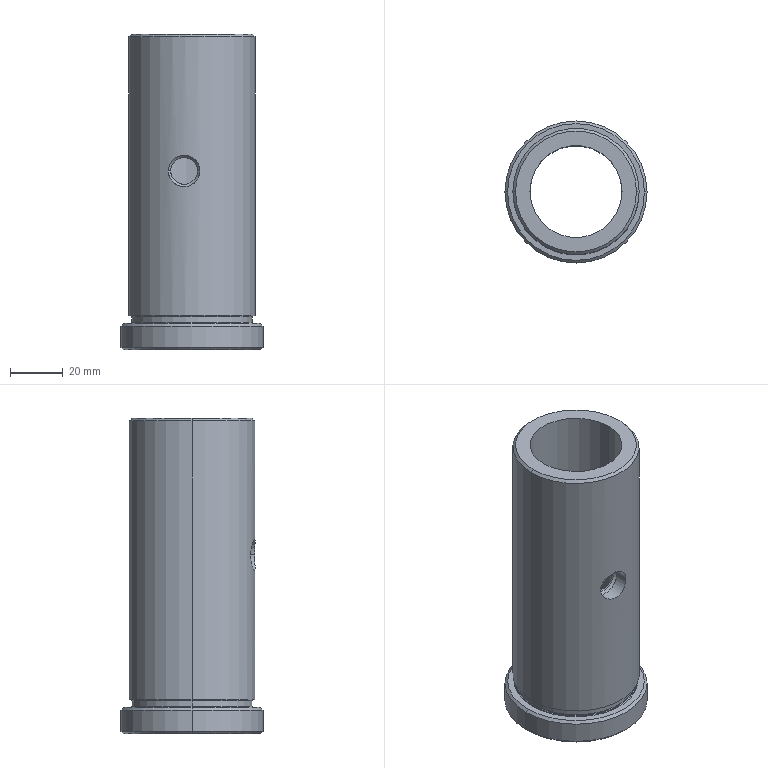Part | Creo | 1 solid | 32 faces | box 54 x 54 x 120 mm | volume 105135 mm3 | cylinder 12 | cone 8 | torus 8 | plane 4 | commonest cylinder face diameters 10.2 x2 12 x2 35 x2 46 x2 48 x2 54 x2
STEP:
#1=CARTESIAN_POINT('',(0.,0.,0.));
#2=DIRECTION('',(0.,0.,1.));
#3=DIRECTION('',(1.,0.,0.));
#4=AXIS2_PLACEMENT_3D('',#1,#2,#3);
#5=CARTESIAN_POINT('',(-189.,-212.,-111.5));
#6=VERTEX_POINT('',#5);
#7=CARTESIAN_POINT('',(-135.,-212.,-111.5));
#8=VERTEX_POINT('',#7);
#9=CARTESIAN_POINT('',(-162.,-212.,-111.5));
#10=DIRECTION('',(0.,0.,1.));
#11=DIRECTION('',(-1.,0.,0.));
#12=AXIS2_PLACEMENT_3D('',#9,#10,#11);
#13=CIRCLE('',#12,27.);
#14=EDGE_CURVE('',#6,#8,#13,.T.);
#15=ORIENTED_EDGE('',*,*,#14,.T.);
#16=CARTESIAN_POINT('',(-135.,-212.,-119.5));
#17=VERTEX_POINT('',#16);
#18=CARTESIAN_POINT('',(-135.,-212.,-111.5));
#19=DIRECTION('',(0.,0.,-1.));
#20=VECTOR('',#19,8.);
#21=LINE('',#18,#20);
#22=EDGE_CURVE('',#8,#17,#21,.T.);
#23=ORIENTED_EDGE('',*,*,#22,.T.);
#24=CARTESIAN_POINT('',(-189.,-212.,-119.5));
#25=VERTEX_POINT('',#24);
#26=CARTESIAN_POINT('',(-162.,-212.,-119.5));
#27=DIRECTION('',(0.,0.,-1.));
#28=DIRECTION('',(1.,0.,0.));
#29=AXIS2_PLACEMENT_3D('',#26,#27,#28);
#30=CIRCLE('',#29,27.);
#31=EDGE_CURVE('',#17,#25,#30,.T.);
#32=ORIENTED_EDGE('',*,*,#31,.T.);
#33=CARTESIAN_POINT('',(-189.,-212.,-111.5));
#34=DIRECTION('',(0.,0.,-1.));
#35=VECTOR('',#34,8.);
#36=LINE('',#33,#35);
#37=EDGE_CURVE('',#6,#25,#36,.T.);
#38=ORIENTED_EDGE('',*,*,#37,.F.);
#39=EDGE_LOOP('',(#15,#23,#32,#38));
#40=FACE_OUTER_BOUND('',#39,.F.);
#41=CARTESIAN_POINT('',(-162.,-212.,-110.5));
#42=DIRECTION('',(0.,0.,-1.));
#43=DIRECTION('',(1.,0.,0.));
#44=AXIS2_PLACEMENT_3D('',#41,#42,#43);
#45=CYLINDRICAL_SURFACE('',#44,27.);
#46=ADVANCED_FACE('',(#40),#45,.T.);
#47=CARTESIAN_POINT('',(-188.,-212.,-110.5));
#48=VERTEX_POINT('',#47);
#49=CARTESIAN_POINT('',(-136.,-212.,-110.5));
#50=VERTEX_POINT('',#49);
#51=CARTESIAN_POINT('',(-162.,-212.,-110.5));
#52=DIRECTION('',(0.,0.,1.));
#53=DIRECTION('',(-1.,0.,0.));
#54=AXIS2_PLACEMENT_3D('',#51,#52,#53);
#55=CIRCLE('',#54,26.);
#56=EDGE_CURVE('',#48,#50,#55,.T.);
#57=ORIENTED_EDGE('',*,*,#56,.T.);
#58=CARTESIAN_POINT('',(-136.,-212.,-110.5));
#59=DIRECTION('',(0.7071,0.,-0.7071));
#60=VECTOR('',#59,1.414);
#61=LINE('',#58,#60);
#62=EDGE_CURVE('',#50,#8,#61,.T.);
#63=ORIENTED_EDGE('',*,*,#62,.T.);
#64=ORIENTED_EDGE('',*,*,#14,.F.);
#65=CARTESIAN_POINT('',(-188.,-212.,-110.5));
#66=DIRECTION('',(-0.7071,0.,-0.7071));
#67=VECTOR('',#66,1.414);
#68=LINE('',#65,#67);
#69=EDGE_CURVE('',#48,#6,#68,.T.);
#70=ORIENTED_EDGE('',*,*,#69,.F.);
#71=EDGE_LOOP('',(#57,#63,#64,#70));
#72=FACE_OUTER_BOUND('',#71,.F.);
#73=CARTESIAN_POINT('',(-162.,-212.,-111.));
#74=DIRECTION('',(0.,0.,-1.));
#75=DIRECTION('',(1.,0.,0.));
#76=AXIS2_PLACEMENT_3D('',#73,#74,#75);
#77=CONICAL_SURFACE('',#76,26.5,45.);
#78=ADVANCED_FACE('',(#72),#77,.T.);
#79=ORIENTED_EDGE('',*,*,#56,.F.);
#80=CARTESIAN_POINT('',(-162.,-212.,-110.5));
#81=DIRECTION('',(0.,0.,1.));
#82=DIRECTION('',(1.,0.,0.));
#83=AXIS2_PLACEMENT_3D('',#80,#81,#82);
#84=CIRCLE('',#83,26.);
#85=EDGE_CURVE('',#50,#48,#84,.T.);
#86=ORIENTED_EDGE('',*,*,#85,.F.);
#87=EDGE_LOOP('',(#79,#86));
#88=FACE_OUTER_BOUND('',#87,.F.);
#89=CARTESIAN_POINT('',(-138.5,-212.,-110.5));
#90=VERTEX_POINT('',#89);
#91=CARTESIAN_POINT('',(-185.5,-212.,-110.5));
#92=VERTEX_POINT('',#91);
#93=CARTESIAN_POINT('',(-162.,-212.,-110.5));
#94=DIRECTION('',(0.,0.,-1.));
#95=DIRECTION('',(1.,0.,0.));
#96=AXIS2_PLACEMENT_3D('',#93,#94,#95);
#97=CIRCLE('',#96,23.5);
#98=EDGE_CURVE('',#90,#92,#97,.T.);
#99=ORIENTED_EDGE('',*,*,#98,.F.);
#100=CARTESIAN_POINT('',(-162.,-212.,-110.5));
#101=DIRECTION('',(0.,0.,-1.));
#102=DIRECTION('',(-1.,0.,0.));
#103=AXIS2_PLACEMENT_3D('',#100,#101,#102);
#104=CIRCLE('',#103,23.5);
#105=EDGE_CURVE('',#92,#90,#104,.T.);
#106=ORIENTED_EDGE('',*,*,#105,.F.);
#107=EDGE_LOOP('',(#99,#106));
#108=FACE_BOUND('',#107,.F.);
#109=CARTESIAN_POINT('',(-162.,-212.,-110.5));
#110=DIRECTION('',(0.,0.,-1.));
#111=DIRECTION('',(1.,0.,0.));
#112=AXIS2_PLACEMENT_3D('',#109,#110,#111);
#113=PLANE('',#112);
#114=ADVANCED_FACE('',(#88,#108),#113,.F.);
#115=ORIENTED_EDGE('',*,*,#85,.T.);
#116=ORIENTED_EDGE('',*,*,#69,.T.);
#117=CARTESIAN_POINT('',(-162.,-212.,-111.5));
#118=DIRECTION('',(0.,0.,1.));
#119=DIRECTION('',(1.,0.,0.));
#120=AXIS2_PLACEMENT_3D('',#117,#118,#119);
#121=CIRCLE('',#120,27.);
#122=EDGE_CURVE('',#8,#6,#121,.T.);
#123=ORIENTED_EDGE('',*,*,#122,.F.);
#124=ORIENTED_EDGE('',*,*,#62,.F.);
#125=EDGE_LOOP('',(#115,#116,#123,#124));
#126=FACE_OUTER_BOUND('',#125,.F.);
#127=CARTESIAN_POINT('',(-162.,-212.,-111.));
#128=DIRECTION('',(0.,0.,-1.));
#129=DIRECTION('',(1.,0.,0.));
#130=AXIS2_PLACEMENT_3D('',#127,#128,#129);
#131=CONICAL_SURFACE('',#130,26.5,45.);
#132=ADVANCED_FACE('',(#126),#131,.T.);
#133=ORIENTED_EDGE('',*,*,#122,.T.);
#134=ORIENTED_EDGE('',*,*,#37,.T.);
#135=CARTESIAN_POINT('',(-162.,-212.,-119.5));
#136=DIRECTION('',(0.,0.,-1.));
#137=DIRECTION('',(-1.,0.,0.));
#138=AXIS2_PLACEMENT_3D('',#135,#136,#137);
#139=CIRCLE('',#138,27.);
#140=EDGE_CURVE('',#25,#17,#139,.T.);
#141=ORIENTED_EDGE('',*,*,#140,.T.);
#142=ORIENTED_EDGE('',*,*,#22,.F.);
#143=EDGE_LOOP('',(#133,#134,#141,#142));
#144=FACE_OUTER_BOUND('',#143,.F.);
#145=CARTESIAN_POINT('',(-162.,-212.,-110.5));
#146=DIRECTION('',(0.,0.,-1.));
#147=DIRECTION('',(1.,0.,0.));
#148=AXIS2_PLACEMENT_3D('',#145,#146,#147);
#149=CYLINDRICAL_SURFACE('',#148,27.);
#150=ADVANCED_FACE('',(#144),#149,.T.);
#151=ORIENTED_EDGE('',*,*,#140,.F.);
#152=CARTESIAN_POINT('',(-188.,-212.,-120.5));
#153=VERTEX_POINT('',#152);
#154=CARTESIAN_POINT('',(-188.,-212.,-120.5));
#155=DIRECTION('',(-0.7071,0.,0.7071));
#156=VECTOR('',#155,1.414);
#157=LINE('',#154,#156);
#158=EDGE_CURVE('',#153,#25,#157,.T.);
#159=ORIENTED_EDGE('',*,*,#158,.F.);
#160=CARTESIAN_POINT('',(-136.,-212.,-120.5));
#161=VERTEX_POINT('',#160);
#162=CARTESIAN_POINT('',(-162.,-212.,-120.5));
#163=DIRECTION('',(0.,0.,-1.));
#164=DIRECTION('',(-1.,0.,0.));
#165=AXIS2_PLACEMENT_3D('',#162,#163,#164);
#166=CIRCLE('',#165,26.);
#167=EDGE_CURVE('',#153,#161,#166,.T.);
#168=ORIENTED_EDGE('',*,*,#167,.T.);
#169=CARTESIAN_POINT('',(-136.,-212.,-120.5));
#170=DIRECTION('',(0.7071,0.,0.7071));
#171=VECTOR('',#170,1.414);
#172=LINE('',#169,#171);
#173=EDGE_CURVE('',#161,#17,#172,.T.);
#174=ORIENTED_EDGE('',*,*,#173,.T.);
#175=EDGE_LOOP('',(#151,#159,#168,#174));
#176=FACE_OUTER_BOUND('',#175,.F.);
#177=CARTESIAN_POINT('',(-162.,-212.,-120.));
#178=DIRECTION('',(0.,0.,1.));
#179=DIRECTION('',(-1.,0.,0.));
#180=AXIS2_PLACEMENT_3D('',#177,#178,#179);
#181=CONICAL_SURFACE('',#180,26.5,45.);
#182=ADVANCED_FACE('',(#176),#181,.T.);
#183=ORIENTED_EDGE('',*,*,#31,.F.);
#184=ORIENTED_EDGE('',*,*,#173,.F.);
#185=CARTESIAN_POINT('',(-162.,-212.,-120.5));
#186=DIRECTION('',(0.,0.,-1.));
#187=DIRECTION('',(1.,0.,0.));
#188=AXIS2_PLACEMENT_3D('',#185,#186,#187);
#189=CIRCLE('',#188,26.);
#190=EDGE_CURVE('',#161,#153,#189,.T.);
#191=ORIENTED_EDGE('',*,*,#190,.T.);
#192=ORIENTED_EDGE('',*,*,#158,.T.);
#193=EDGE_LOOP('',(#183,#184,#191,#192));
#194=FACE_OUTER_BOUND('',#193,.F.);
#195=CARTESIAN_POINT('',(-162.,-212.,-120.));
#196=DIRECTION('',(0.,0.,1.));
#197=DIRECTION('',(-1.,0.,0.));
#198=AXIS2_PLACEMENT_3D('',#195,#196,#197);
#199=CONICAL_SURFACE('',#198,26.5,45.);
#200=ADVANCED_FACE('',(#194),#199,.T.);
#201=ORIENTED_EDGE('',*,*,#167,.F.);
#202=ORIENTED_EDGE('',*,*,#190,.F.);
#203=EDGE_LOOP('',(#201,#202));
#204=FACE_OUTER_BOUND('',#203,.F.);
#205=CARTESIAN_POINT('',(-144.5,-212.,-120.5));
#206=VERTEX_POINT('',#205);
#207=CARTESIAN_POINT('',(-179.5,-212.,-120.5));
#208=VERTEX_POINT('',#207);
#209=CARTESIAN_POINT('',(-162.,-212.,-120.5));
#210=DIRECTION('',(0.,0.,1.));
#211=DIRECTION('',(1.,0.,0.));
#212=AXIS2_PLACEMENT_3D('',#209,#210,#211);
#213=CIRCLE('',#212,17.5);
#214=EDGE_CURVE('',#206,#208,#213,.T.);
#215=ORIENTED_EDGE('',*,*,#214,.F.);
#216=CARTESIAN_POINT('',(-162.,-212.,-120.5));
#217=DIRECTION('',(0.,0.,1.));
#218=DIRECTION('',(-1.,0.,0.));
#219=AXIS2_PLACEMENT_3D('',#216,#217,#218);
#220=CIRCLE('',#219,17.5);
#221=EDGE_CURVE('',#208,#206,#220,.T.);
#222=ORIENTED_EDGE('',*,*,#221,.F.);
#223=EDGE_LOOP('',(#215,#222));
#224=FACE_BOUND('',#223,.F.);
#225=CARTESIAN_POINT('',(-162.,-212.,-120.5));
#226=DIRECTION('',(0.,0.,-1.));
#227=DIRECTION('',(1.,0.,0.));
#228=AXIS2_PLACEMENT_3D('',#225,#226,#227);
#229=PLANE('',#228);
#230=ADVANCED_FACE('',(#204,#224),#229,.T.);
#231=CARTESIAN_POINT('',(-179.5,-212.,-0.5));
#232=VERTEX_POINT('',#231);
#233=CARTESIAN_POINT('',(-144.5,-212.,-0.5));
#234=VERTEX_POINT('',#233);
#235=CARTESIAN_POINT('',(-162.,-212.,-0.5));
#236=DIRECTION('',(0.,0.,-1.));
#237=DIRECTION('',(-1.,0.,0.));
#238=AXIS2_PLACEMENT_3D('',#235,#236,#237);
#239=CIRCLE('',#238,17.5);
#240=EDGE_CURVE('',#232,#234,#239,.T.);
#241=ORIENTED_EDGE('',*,*,#240,.T.);
#242=CARTESIAN_POINT('',(-144.5,-212.,-120.5));
#243=DIRECTION('',(0.,0.,1.));
#244=VECTOR('',#243,120.);
#245=LINE('',#242,#244);
#246=EDGE_CURVE('',#206,#234,#245,.T.);
#247=ORIENTED_EDGE('',*,*,#246,.F.);
#248=ORIENTED_EDGE('',*,*,#214,.T.);
#249=CARTESIAN_POINT('',(-179.5,-212.,-120.5));
#250=DIRECTION('',(0.,0.,1.));
#251=VECTOR('',#250,120.);
#252=LINE('',#249,#251);
#253=EDGE_CURVE('',#208,#232,#252,.T.);
#254=ORIENTED_EDGE('',*,*,#253,.T.);
#255=EDGE_LOOP('',(#241,#247,#248,#254));
#256=FACE_OUTER_BOUND('',#255,.F.);
#257=CARTESIAN_POINT('',(-162.,-212.,-120.5));
#258=DIRECTION('',(0.,0.,1.));
#259=DIRECTION('',(-1.,0.,0.));
#260=AXIS2_PLACEMENT_3D('',#257,#258,#259);
#261=CYLINDRICAL_SURFACE('',#260,17.5);
#262=ADVANCED_FACE('',(#256),#261,.F.);
#263=CARTESIAN_POINT('',(-139.,-212.,-0.5));
#264=VERTEX_POINT('',#263);
#265=CARTESIAN_POINT('',(-185.,-212.,-0.5));
#266=VERTEX_POINT('',#265);
#267=CARTESIAN_POINT('',(-162.,-212.,-0.5));
#268=DIRECTION('',(0.,0.,1.));
#269=DIRECTION('',(1.,0.,0.));
#270=AXIS2_PLACEMENT_3D('',#267,#268,#269);
#271=CIRCLE('',#270,23.);
#272=EDGE_CURVE('',#264,#266,#271,.T.);
#273=ORIENTED_EDGE('',*,*,#272,.F.);
#274=CARTESIAN_POINT('',(-162.,-212.,-0.5));
#275=DIRECTION('',(0.,0.,1.));
#276=DIRECTION('',(-1.,0.,0.));
#277=AXIS2_PLACEMENT_3D('',#274,#275,#276);
#278=CIRCLE('',#277,23.);
#279=EDGE_CURVE('',#266,#264,#278,.T.);
#280=ORIENTED_EDGE('',*,*,#279,.F.);
#281=EDGE_LOOP('',(#273,#280));
#282=FACE_OUTER_BOUND('',#281,.F.);
#283=CARTESIAN_POINT('',(-162.,-212.,-0.5));
#284=DIRECTION('',(0.,0.,-1.));
#285=DIRECTION('',(1.,0.,0.));
#286=AXIS2_PLACEMENT_3D('',#283,#284,#285);
#287=CIRCLE('',#286,17.5);
#288=EDGE_CURVE('',#234,#232,#287,.T.);
#289=ORIENTED_EDGE('',*,*,#288,.F.);
#290=ORIENTED_EDGE('',*,*,#240,.F.);
#291=EDGE_LOOP('',(#289,#290));
#292=FACE_BOUND('',#291,.F.);
#293=CARTESIAN_POINT('',(-162.,-212.,-0.5));
#294=DIRECTION('',(0.,0.,1.));
#295=DIRECTION('',(-1.,0.,0.));
#296=AXIS2_PLACEMENT_3D('',#293,#294,#295);
#297=PLANE('',#296);
#298=ADVANCED_FACE('',(#282,#292),#297,.T.);
#299=ORIENTED_EDGE('',*,*,#288,.T.);
#300=ORIENTED_EDGE('',*,*,#253,.F.);
#301=ORIENTED_EDGE('',*,*,#221,.T.);
#302=ORIENTED_EDGE('',*,*,#246,.T.);
#303=EDGE_LOOP('',(#299,#300,#301,#302));
#304=FACE_OUTER_BOUND('',#303,.F.);
#305=CARTESIAN_POINT('',(-159.9,-229.374,-52.5));
#306=VERTEX_POINT('',#305);
#307=CARTESIAN_POINT('',(-170.1,-227.513,-52.5));
#308=VERTEX_POINT('',#307);
#309=CARTESIAN_POINT('',(-159.9,-229.374,-52.5));
#310=CARTESIAN_POINT('',(-159.9,-229.374,-52.883));
#311=CARTESIAN_POINT('',(-159.986,-229.384,-53.65));
#312=CARTESIAN_POINT('',(-160.375,-229.427,-54.754));
#313=CARTESIAN_POINT('',(-161.008,-229.477,-55.743));
#314=CARTESIAN_POINT('',(-161.827,-229.507,-56.548));
#315=CARTESIAN_POINT('',(-162.814,-229.492,-57.156));
#316=CARTESIAN_POINT('',(-163.903,-229.408,-57.524));
#317=CARTESIAN_POINT('',(-165.043,-229.246,-57.642));
#318=CARTESIAN_POINT('',(-166.188,-229.005,-57.505));
#319=CARTESIAN_POINT('',(-167.292,-228.693,-57.107));
#320=CARTESIAN_POINT('',(-168.281,-228.344,-56.462));
#321=CARTESIAN_POINT('',(-169.086,-228.007,-55.625));
#322=CARTESIAN_POINT('',(-169.686,-227.725,-54.621));
#323=CARTESIAN_POINT('',(-170.032,-227.549,-53.544));
#324=CARTESIAN_POINT('',(-170.1,-227.513,-52.841));
#325=CARTESIAN_POINT('',(-170.1,-227.513,-52.5));
#326=B_SPLINE_CURVE_WITH_KNOTS('',3,(#309,#310,#311,#312,#313,#314,#315,#316,#317,#318,#319,#320,#321,#322,#323,#324,#325),.UNSPECIFIED.,.F.,.F.,(4,1,1,1,1,1,1,1,1,1,1,1,1,1,4),(0.,0.07143,0.1429,0.2143,0.2857,0.3571,0.4286,0.5,0.5714,0.6429,0.7143,0.7857,0.8571,0.9286,1.),.UNSPECIFIED.);
#327=EDGE_CURVE('',#306,#308,#326,.T.);
#328=ORIENTED_EDGE('',*,*,#327,.T.);
#329=CARTESIAN_POINT('',(-170.1,-227.513,-52.5));
#330=CARTESIAN_POINT('',(-170.1,-227.513,-52.158));
#331=CARTESIAN_POINT('',(-170.031,-227.549,-51.456));
#332=CARTESIAN_POINT('',(-169.689,-227.723,-50.388));
#333=CARTESIAN_POINT('',(-169.099,-228.001,-49.393));
#334=CARTESIAN_POINT('',(-168.303,-228.335,-48.556));
#335=CARTESIAN_POINT('',(-167.317,-228.685,-47.905));
#336=CARTESIAN_POINT('',(-166.207,-229.,-47.499));
#337=CARTESIAN_POINT('',(-165.06,-229.244,-47.358));
#338=CARTESIAN_POINT('',(-163.922,-229.406,-47.472));
#339=CARTESIAN_POINT('',(-162.838,-229.49,-47.834));
#340=CARTESIAN_POINT('',(-161.851,-229.507,-48.434));
#341=CARTESIAN_POINT('',(-161.022,-229.478,-49.239));
#342=CARTESIAN_POINT('',(-160.38,-229.427,-50.234));
#343=CARTESIAN_POINT('',(-159.986,-229.384,-51.349));
#344=CARTESIAN_POINT('',(-159.9,-229.374,-52.119));
#345=CARTESIAN_POINT('',(-159.9,-229.374,-52.5));
#346=B_SPLINE_CURVE_WITH_KNOTS('',3,(#329,#330,#331,#332,#333,#334,#335,#336,#337,#338,#339,#340,#341,#342,#343,#344,#345),.UNSPECIFIED.,.F.,.F.,(4,1,1,1,1,1,1,1,1,1,1,1,1,1,4),(0.,0.07143,0.1429,0.2143,0.2857,0.3571,0.4286,0.5,0.5714,0.6429,0.7143,0.7857,0.8571,0.9286,1.),.UNSPECIFIED.);
#347=EDGE_CURVE('',#308,#306,#346,.T.);
#348=ORIENTED_EDGE('',*,*,#347,.T.);
#349=EDGE_LOOP('',(#328,#348));
#350=FACE_BOUND('',#349,.F.);
#351=CARTESIAN_POINT('',(-162.,-212.,-120.5));
#352=DIRECTION('',(0.,0.,1.));
#353=DIRECTION('',(-1.,0.,0.));
#354=AXIS2_PLACEMENT_3D('',#351,#352,#353);
#355=CYLINDRICAL_SURFACE('',#354,17.5);
#356=ADVANCED_FACE('',(#304,#350),#355,.F.);
#357=CARTESIAN_POINT('',(-159.9,-230.1,-52.5));
#358=VERTEX_POINT('',#357);
#359=CARTESIAN_POINT('',(-170.1,-230.1,-52.5));
#360=VERTEX_POINT('',#359);
#361=CARTESIAN_POINT('',(-165.,-230.1,-52.5));
#362=DIRECTION('',(0.,1.,0.));
#363=DIRECTION('',(1.,0.,0.));
#364=AXIS2_PLACEMENT_3D('',#361,#362,#363);
#365=CIRCLE('',#364,5.1);
#366=EDGE_CURVE('',#358,#360,#365,.T.);
#367=ORIENTED_EDGE('',*,*,#366,.T.);
#368=CARTESIAN_POINT('',(-170.1,-227.513,-52.5));
#369=DIRECTION('',(0.,-1.,0.));
#370=VECTOR('',#369,2.587);
#371=LINE('',#368,#370);
#372=EDGE_CURVE('',#308,#360,#371,.T.);
#373=ORIENTED_EDGE('',*,*,#372,.F.);
#374=ORIENTED_EDGE('',*,*,#327,.F.);
#375=CARTESIAN_POINT('',(-159.9,-229.374,-52.5));
#376=DIRECTION('',(0.00000007,-1.,0.000573));
#377=VECTOR('',#376,0.7265);
#378=LINE('',#375,#377);
#379=EDGE_CURVE('',#306,#358,#378,.T.);
#380=ORIENTED_EDGE('',*,*,#379,.T.);
#381=EDGE_LOOP('',(#367,#373,#374,#380));
#382=FACE_OUTER_BOUND('',#381,.F.);
#383=CARTESIAN_POINT('',(-165.,-300.,-52.5));
#384=DIRECTION('',(0.,-1.,0.));
#385=DIRECTION('',(-1.,0.,0.));
#386=AXIS2_PLACEMENT_3D('',#383,#384,#385);
#387=CYLINDRICAL_SURFACE('',#386,5.1);
#388=ADVANCED_FACE('',(#382),#387,.F.);
#389=ORIENTED_EDGE('',*,*,#366,.F.);
#390=CARTESIAN_POINT('',(-159.,-231.,-52.5));
#391=VERTEX_POINT('',#390);
#392=CARTESIAN_POINT('',(-159.9,-230.1,-52.5));
#393=DIRECTION('',(0.7071,-0.7071,0.));
#394=VECTOR('',#393,1.273);
#395=LINE('',#392,#394);
#396=EDGE_CURVE('',#358,#391,#395,.T.);
#397=ORIENTED_EDGE('',*,*,#396,.T.);
#398=CARTESIAN_POINT('',(-171.,-231.,-52.5));
#399=VERTEX_POINT('',#398);
#400=CARTESIAN_POINT('',(-165.,-231.,-52.5));
#401=DIRECTION('',(0.,-1.,0.));
#402=DIRECTION('',(-1.,0.,0.));
#403=AXIS2_PLACEMENT_3D('',#400,#401,#402);
#404=CIRCLE('',#403,6.);
#405=EDGE_CURVE('',#399,#391,#404,.T.);
#406=ORIENTED_EDGE('',*,*,#405,.F.);
#407=CARTESIAN_POINT('',(-170.1,-230.1,-52.5));
#408=DIRECTION('',(-0.7071,-0.7071,0.));
#409=VECTOR('',#408,1.273);
#410=LINE('',#407,#409);
#411=EDGE_CURVE('',#360,#399,#410,.T.);
#412=ORIENTED_EDGE('',*,*,#411,.F.);
#413=EDGE_LOOP('',(#389,#397,#406,#412));
#414=FACE_OUTER_BOUND('',#413,.F.);
#415=CARTESIAN_POINT('',(-165.,-230.55,-52.5));
#416=DIRECTION('',(0.,-1.,0.));
#417=DIRECTION('',(-1.,0.,0.));
#418=AXIS2_PLACEMENT_3D('',#415,#416,#417);
#419=CONICAL_SURFACE('',#418,5.55,45.);
#420=ADVANCED_FACE('',(#414),#419,.F.);
#421=CARTESIAN_POINT('',(-165.,-230.1,-52.5));
#422=DIRECTION('',(0.,1.,0.));
#423=DIRECTION('',(-1.,0.,0.));
#424=AXIS2_PLACEMENT_3D('',#421,#422,#423);
#425=CIRCLE('',#424,5.1);
#426=EDGE_CURVE('',#360,#358,#425,.T.);
#427=ORIENTED_EDGE('',*,*,#426,.F.);
#428=ORIENTED_EDGE('',*,*,#411,.T.);
#429=CARTESIAN_POINT('',(-165.,-231.,-52.5));
#430=DIRECTION('',(0.,-1.,0.));
#431=DIRECTION('',(1.,0.,0.));
#432=AXIS2_PLACEMENT_3D('',#429,#430,#431);
#433=CIRCLE('',#432,6.);
#434=EDGE_CURVE('',#391,#399,#433,.T.);
#435=ORIENTED_EDGE('',*,*,#434,.F.);
#436=ORIENTED_EDGE('',*,*,#396,.F.);
#437=EDGE_LOOP('',(#427,#428,#435,#436));
#438=FACE_OUTER_BOUND('',#437,.F.);
#439=CARTESIAN_POINT('',(-165.,-230.55,-52.5));
#440=DIRECTION('',(0.,-1.,0.));
#441=DIRECTION('',(-1.,0.,0.));
#442=AXIS2_PLACEMENT_3D('',#439,#440,#441);
#443=CONICAL_SURFACE('',#442,5.55,45.);
#444=ADVANCED_FACE('',(#438),#443,.F.);
#445=ORIENTED_EDGE('',*,*,#426,.T.);
#446=ORIENTED_EDGE('',*,*,#379,.F.);
#447=ORIENTED_EDGE('',*,*,#347,.F.);
#448=ORIENTED_EDGE('',*,*,#372,.T.);
#449=EDGE_LOOP('',(#445,#446,#447,#448));
#450=FACE_OUTER_BOUND('',#449,.F.);
#451=CARTESIAN_POINT('',(-165.,-300.,-52.5));
#452=DIRECTION('',(0.,-1.,0.));
#453=DIRECTION('',(-1.,0.,0.));
#454=AXIS2_PLACEMENT_3D('',#451,#452,#453);
#455=CYLINDRICAL_SURFACE('',#454,5.1);
#456=ADVANCED_FACE('',(#450),#455,.F.);
#457=CARTESIAN_POINT('',(-171.,-234.249,-52.5));
#458=VERTEX_POINT('',#457);
#459=CARTESIAN_POINT('',(-159.,-235.812,-52.501));
#460=VERTEX_POINT('',#459);
#461=CARTESIAN_POINT('',(-171.,-234.249,-52.5));
#462=CARTESIAN_POINT('',(-171.,-234.249,-52.07));
#463=CARTESIAN_POINT('',(-170.911,-234.285,-51.222));
#464=CARTESIAN_POINT('',(-170.485,-234.453,-49.943));
#465=CARTESIAN_POINT('',(-169.772,-234.713,-48.779));
#466=CARTESIAN_POINT('',(-168.819,-235.02,-47.806));
#467=CARTESIAN_POINT('',(-167.66,-235.335,-47.063));
#468=CARTESIAN_POINT('',(-166.358,-235.614,-46.602));
#469=CARTESIAN_POINT('',(-164.999,-235.825,-46.449));
#470=CARTESIAN_POINT('',(-163.646,-235.956,-46.603));
#471=CARTESIAN_POINT('',(-162.366,-236.008,-47.053));
#472=CARTESIAN_POINT('',(-161.221,-235.995,-47.776));
#473=CARTESIAN_POINT('',(-160.271,-235.943,-48.726));
#474=CARTESIAN_POINT('',(-159.544,-235.876,-49.88));
#475=CARTESIAN_POINT('',(-159.098,-235.824,-51.173));
#476=CARTESIAN_POINT('',(-159.,-235.812,-52.05));
#477=CARTESIAN_POINT('',(-159.,-235.812,-52.501));
#478=B_SPLINE_CURVE_WITH_KNOTS('',3,(#461,#462,#463,#464,#465,#466,#467,#468,#469,#470,#471,#472,#473,#474,#475,#476,#477),.UNSPECIFIED.,.F.,.F.,(4,1,1,1,1,1,1,1,1,1,1,1,1,1,4),(0.,0.07143,0.1429,0.2143,0.2857,0.3571,0.4286,0.5,0.5714,0.6429,0.7143,0.7857,0.8571,0.9286,1.),.UNSPECIFIED.);
#479=EDGE_CURVE('',#458,#460,#478,.T.);
#480=ORIENTED_EDGE('',*,*,#479,.T.);
#481=CARTESIAN_POINT('',(-159.,-231.,-52.5));
#482=DIRECTION('',(-0.000000014,-1.,-0.0001098));
#483=VECTOR('',#482,4.812);
#484=LINE('',#481,#483);
#485=EDGE_CURVE('',#391,#460,#484,.T.);
#486=ORIENTED_EDGE('',*,*,#485,.F.);
#487=ORIENTED_EDGE('',*,*,#434,.T.);
#488=CARTESIAN_POINT('',(-171.,-231.,-52.5));
#489=DIRECTION('',(0.,-1.,0.));
#490=VECTOR('',#489,3.249);
#491=LINE('',#488,#490);
#492=EDGE_CURVE('',#399,#458,#491,.T.);
#493=ORIENTED_EDGE('',*,*,#492,.T.);
#494=EDGE_LOOP('',(#480,#486,#487,#493));
#495=FACE_OUTER_BOUND('',#494,.F.);
#496=CARTESIAN_POINT('',(-165.,-300.,-52.5));
#497=DIRECTION('',(0.,-1.,0.));
#498=DIRECTION('',(-1.,0.,0.));
#499=AXIS2_PLACEMENT_3D('',#496,#497,#498);
#500=CYLINDRICAL_SURFACE('',#499,6.);
#501=ADVANCED_FACE('',(#495),#500,.F.);
#502=CARTESIAN_POINT('',(-138.,-212.,-107.5));
#503=VERTEX_POINT('',#502);
#504=CARTESIAN_POINT('',(-186.,-212.,-107.5));
#505=VERTEX_POINT('',#504);
#506=CARTESIAN_POINT('',(-162.,-212.,-107.5));
#507=DIRECTION('',(0.,0.,-1.));
#508=DIRECTION('',(1.,0.,0.));
#509=AXIS2_PLACEMENT_3D('',#506,#507,#508);
#510=CIRCLE('',#509,24.);
#511=EDGE_CURVE('',#503,#505,#510,.T.);
#512=ORIENTED_EDGE('',*,*,#511,.T.);
#513=CARTESIAN_POINT('',(-186.,-212.,-1.5));
#514=VERTEX_POINT('',#513);
#515=CARTESIAN_POINT('',(-186.,-212.,-107.5));
#516=DIRECTION('',(0.,0.,1.));
#517=VECTOR('',#516,106.);
#518=LINE('',#515,#517);
#519=EDGE_CURVE('',#505,#514,#518,.T.);
#520=ORIENTED_EDGE('',*,*,#519,.T.);
#521=CARTESIAN_POINT('',(-138.,-212.,-1.5));
#522=VERTEX_POINT('',#521);
#523=CARTESIAN_POINT('',(-162.,-212.,-1.5));
#524=DIRECTION('',(0.,0.,1.));
#525=DIRECTION('',(-1.,0.,0.));
#526=AXIS2_PLACEMENT_3D('',#523,#524,#525);
#527=CIRCLE('',#526,24.);
#528=EDGE_CURVE('',#514,#522,#527,.T.);
#529=ORIENTED_EDGE('',*,*,#528,.T.);
#530=CARTESIAN_POINT('',(-138.,-212.,-107.5));
#531=DIRECTION('',(0.,0.,1.));
#532=VECTOR('',#531,106.);
#533=LINE('',#530,#532);
#534=EDGE_CURVE('',#503,#522,#533,.T.);
#535=ORIENTED_EDGE('',*,*,#534,.F.);
#536=EDGE_LOOP('',(#512,#520,#529,#535));
#537=FACE_OUTER_BOUND('',#536,.F.);
#538=ORIENTED_EDGE('',*,*,#479,.F.);
#539=CARTESIAN_POINT('',(-159.,-235.812,-52.501));
#540=CARTESIAN_POINT('',(-159.,-235.812,-52.95));
#541=CARTESIAN_POINT('',(-159.099,-235.824,-53.828));
#542=CARTESIAN_POINT('',(-159.539,-235.876,-55.107));
#543=CARTESIAN_POINT('',(-160.258,-235.942,-56.257));
#544=CARTESIAN_POINT('',(-161.198,-235.994,-57.206));
#545=CARTESIAN_POINT('',(-162.349,-236.008,-57.94));
#546=CARTESIAN_POINT('',(-163.632,-235.957,-58.394));
#547=CARTESIAN_POINT('',(-164.985,-235.827,-58.551));
#548=CARTESIAN_POINT('',(-166.34,-235.617,-58.401));
#549=CARTESIAN_POINT('',(-167.637,-235.34,-57.948));
#550=CARTESIAN_POINT('',(-168.801,-235.025,-57.209));
#551=CARTESIAN_POINT('',(-169.761,-234.716,-56.236));
#552=CARTESIAN_POINT('',(-170.481,-234.454,-55.066));
#553=CARTESIAN_POINT('',(-170.911,-234.285,-53.779));
#554=CARTESIAN_POINT('',(-171.,-234.249,-52.93));
#555=CARTESIAN_POINT('',(-171.,-234.249,-52.5));
#556=B_SPLINE_CURVE_WITH_KNOTS('',3,(#539,#540,#541,#542,#543,#544,#545,#546,#547,#548,#549,#550,#551,#552,#553,#554,#555),.UNSPECIFIED.,.F.,.F.,(4,1,1,1,1,1,1,1,1,1,1,1,1,1,4),(0.,0.07143,0.1429,0.2143,0.2857,0.3571,0.4286,0.5,0.5714,0.6429,0.7143,0.7857,0.8571,0.9286,1.),.UNSPECIFIED.);
#557=EDGE_CURVE('',#460,#458,#556,.T.);
#558=ORIENTED_EDGE('',*,*,#557,.F.);
#559=EDGE_LOOP('',(#538,#558));
#560=FACE_BOUND('',#559,.F.);
#561=CARTESIAN_POINT('',(-162.,-212.,-110.5));
#562=DIRECTION('',(0.,0.,1.));
#563=DIRECTION('',(-1.,0.,0.));
#564=AXIS2_PLACEMENT_3D('',#561,#562,#563);
#565=CYLINDRICAL_SURFACE('',#564,24.);
#566=ADVANCED_FACE('',(#537,#560),#565,.T.);
#567=ORIENTED_EDGE('',*,*,#557,.T.);
#568=ORIENTED_EDGE('',*,*,#492,.F.);
#569=ORIENTED_EDGE('',*,*,#405,.T.);
#570=ORIENTED_EDGE('',*,*,#485,.T.);
#571=EDGE_LOOP('',(#567,#568,#569,#570));
#572=FACE_OUTER_BOUND('',#571,.F.);
#573=CARTESIAN_POINT('',(-165.,-300.,-52.5));
#574=DIRECTION('',(0.,-1.,0.));
#575=DIRECTION('',(-1.,0.,0.));
#576=AXIS2_PLACEMENT_3D('',#573,#574,#575);
#577=CYLINDRICAL_SURFACE('',#576,6.);
#578=ADVANCED_FACE('',(#572),#577,.F.);
#579=ORIENTED_EDGE('',*,*,#511,.F.);
#580=CARTESIAN_POINT('',(-162.,-212.,-107.5));
#581=DIRECTION('',(0.,0.,-1.));
#582=DIRECTION('',(-1.,0.,0.));
#583=AXIS2_PLACEMENT_3D('',#580,#581,#582);
#584=CIRCLE('',#583,24.);
#585=EDGE_CURVE('',#505,#503,#584,.T.);
#586=ORIENTED_EDGE('',*,*,#585,.F.);
#587=EDGE_LOOP('',(#579,#586));
#588=FACE_OUTER_BOUND('',#587,.F.);
#589=CARTESIAN_POINT('',(-138.5,-212.,-107.5));
#590=VERTEX_POINT('',#589);
#591=CARTESIAN_POINT('',(-185.5,-212.,-107.5));
#592=VERTEX_POINT('',#591);
#593=CARTESIAN_POINT('',(-162.,-212.,-107.5));
#594=DIRECTION('',(0.,0.,1.));
#595=DIRECTION('',(1.,0.,0.));
#596=AXIS2_PLACEMENT_3D('',#593,#594,#595);
#597=CIRCLE('',#596,23.5);
#598=EDGE_CURVE('',#590,#592,#597,.T.);
#599=ORIENTED_EDGE('',*,*,#598,.F.);
#600=CARTESIAN_POINT('',(-162.,-212.,-107.5));
#601=DIRECTION('',(0.,0.,1.));
#602=DIRECTION('',(-1.,0.,0.));
#603=AXIS2_PLACEMENT_3D('',#600,#601,#602);
#604=CIRCLE('',#603,23.5);
#605=EDGE_CURVE('',#592,#590,#604,.T.);
#606=ORIENTED_EDGE('',*,*,#605,.F.);
#607=EDGE_LOOP('',(#599,#606));
#608=FACE_BOUND('',#607,.F.);
#609=CARTESIAN_POINT('',(-162.,-212.,-107.5));
#610=DIRECTION('',(0.,0.,1.));
#611=DIRECTION('',(-1.,0.,0.));
#612=AXIS2_PLACEMENT_3D('',#609,#610,#611);
#613=PLANE('',#612);
#614=ADVANCED_FACE('',(#588,#608),#613,.F.);
#615=ORIENTED_EDGE('',*,*,#585,.T.);
#616=ORIENTED_EDGE('',*,*,#534,.T.);
#617=CARTESIAN_POINT('',(-162.,-212.,-1.5));
#618=DIRECTION('',(0.,0.,1.));
#619=DIRECTION('',(1.,0.,0.));
#620=AXIS2_PLACEMENT_3D('',#617,#618,#619);
#621=CIRCLE('',#620,24.);
#622=EDGE_CURVE('',#522,#514,#621,.T.);
#623=ORIENTED_EDGE('',*,*,#622,.T.);
#624=ORIENTED_EDGE('',*,*,#519,.F.);
#625=EDGE_LOOP('',(#615,#616,#623,#624));
#626=FACE_OUTER_BOUND('',#625,.F.);
#627=CARTESIAN_POINT('',(-162.,-212.,-110.5));
#628=DIRECTION('',(0.,0.,1.));
#629=DIRECTION('',(-1.,0.,0.));
#630=AXIS2_PLACEMENT_3D('',#627,#628,#629);
#631=CYLINDRICAL_SURFACE('',#630,24.);
#632=ADVANCED_FACE('',(#626),#631,.T.);
#633=ORIENTED_EDGE('',*,*,#622,.F.);
#634=CARTESIAN_POINT('',(-139.,-212.,-0.5));
#635=DIRECTION('',(0.7071,0.,-0.7071));
#636=VECTOR('',#635,1.414);
#637=LINE('',#634,#636);
#638=EDGE_CURVE('',#264,#522,#637,.T.);
#639=ORIENTED_EDGE('',*,*,#638,.F.);
#640=ORIENTED_EDGE('',*,*,#272,.T.);
#641=CARTESIAN_POINT('',(-185.,-212.,-0.5));
#642=DIRECTION('',(-0.7071,0.,-0.7071));
#643=VECTOR('',#642,1.414);
#644=LINE('',#641,#643);
#645=EDGE_CURVE('',#266,#514,#644,.T.);
#646=ORIENTED_EDGE('',*,*,#645,.T.);
#647=EDGE_LOOP('',(#633,#639,#640,#646));
#648=FACE_OUTER_BOUND('',#647,.F.);
#649=CARTESIAN_POINT('',(-162.,-212.,-1.));
#650=DIRECTION('',(0.,0.,-1.));
#651=DIRECTION('',(1.,0.,0.));
#652=AXIS2_PLACEMENT_3D('',#649,#650,#651);
#653=CONICAL_SURFACE('',#652,23.5,45.);
#654=ADVANCED_FACE('',(#648),#653,.T.);
#655=ORIENTED_EDGE('',*,*,#528,.F.);
#656=ORIENTED_EDGE('',*,*,#645,.F.);
#657=ORIENTED_EDGE('',*,*,#279,.T.);
#658=ORIENTED_EDGE('',*,*,#638,.T.);
#659=EDGE_LOOP('',(#655,#656,#657,#658));
#660=FACE_OUTER_BOUND('',#659,.F.);
#661=CARTESIAN_POINT('',(-162.,-212.,-1.));
#662=DIRECTION('',(0.,0.,-1.));
#663=DIRECTION('',(1.,0.,0.));
#664=AXIS2_PLACEMENT_3D('',#661,#662,#663);
#665=CONICAL_SURFACE('',#664,23.5,45.);
#666=ADVANCED_FACE('',(#660),#665,.T.);
#667=ORIENTED_EDGE('',*,*,#598,.T.);
#668=CARTESIAN_POINT('',(-185.146,-212.,-107.646));
#669=VERTEX_POINT('',#668);
#670=CARTESIAN_POINT('',(-185.5,-212.,-108.));
#671=DIRECTION('',(0.,1.,0.));
#672=DIRECTION('',(0.,0.,1.));
#673=AXIS2_PLACEMENT_3D('',#670,#671,#672);
#674=CIRCLE('',#673,0.5);
#675=EDGE_CURVE('',#592,#669,#674,.T.);
#676=ORIENTED_EDGE('',*,*,#675,.T.);
#677=CARTESIAN_POINT('',(-138.854,-212.,-107.646));
#678=VERTEX_POINT('',#677);
#679=CARTESIAN_POINT('',(-162.,-212.,-107.646));
#680=DIRECTION('',(0.,0.,1.));
#681=DIRECTION('',(1.,0.,0.));
#682=AXIS2_PLACEMENT_3D('',#679,#680,#681);
#683=CIRCLE('',#682,23.146);
#684=EDGE_CURVE('',#678,#669,#683,.T.);
#685=ORIENTED_EDGE('',*,*,#684,.F.);
#686=CARTESIAN_POINT('',(-138.5,-212.,-108.));
#687=DIRECTION('',(0.,-1.,0.));
#688=DIRECTION('',(0.,0.,1.));
#689=AXIS2_PLACEMENT_3D('',#686,#687,#688);
#690=CIRCLE('',#689,0.5);
#691=EDGE_CURVE('',#590,#678,#690,.T.);
#692=ORIENTED_EDGE('',*,*,#691,.F.);
#693=EDGE_LOOP('',(#667,#676,#685,#692));
#694=FACE_OUTER_BOUND('',#693,.F.);
#695=CARTESIAN_POINT('',(-162.,-212.,-108.));
#696=DIRECTION('',(0.,0.,1.));
#697=DIRECTION('',(-1.,0.,0.));
#698=AXIS2_PLACEMENT_3D('',#695,#696,#697);
#699=TOROIDAL_SURFACE('',#698,23.5,0.5);
#700=ADVANCED_FACE('',(#694),#699,.F.);
#701=ORIENTED_EDGE('',*,*,#605,.T.);
#702=ORIENTED_EDGE('',*,*,#691,.T.);
#703=CARTESIAN_POINT('',(-162.,-212.,-107.646));
#704=DIRECTION('',(0.,0.,1.));
#705=DIRECTION('',(-1.,0.,0.));
#706=AXIS2_PLACEMENT_3D('',#703,#704,#705);
#707=CIRCLE('',#706,23.146);
#708=EDGE_CURVE('',#669,#678,#707,.T.);
#709=ORIENTED_EDGE('',*,*,#708,.F.);
#710=ORIENTED_EDGE('',*,*,#675,.F.);
#711=EDGE_LOOP('',(#701,#702,#709,#710));
#712=FACE_OUTER_BOUND('',#711,.F.);
#713=CARTESIAN_POINT('',(-162.,-212.,-108.));
#714=DIRECTION('',(0.,0.,1.));
#715=DIRECTION('',(-1.,0.,0.));
#716=AXIS2_PLACEMENT_3D('',#713,#714,#715);
#717=TOROIDAL_SURFACE('',#716,23.5,0.5);
#718=ADVANCED_FACE('',(#712),#717,.F.);
#719=CARTESIAN_POINT('',(-185.,-212.,-108.));
#720=VERTEX_POINT('',#719);
#721=CARTESIAN_POINT('',(-139.,-212.,-108.));
#722=VERTEX_POINT('',#721);
#723=CARTESIAN_POINT('',(-162.,-212.,-108.));
#724=DIRECTION('',(0.,0.,1.));
#725=DIRECTION('',(-1.,0.,0.));
#726=AXIS2_PLACEMENT_3D('',#723,#724,#725);
#727=CIRCLE('',#726,23.);
#728=EDGE_CURVE('',#720,#722,#727,.T.);
#729=ORIENTED_EDGE('',*,*,#728,.F.);
#730=CARTESIAN_POINT('',(-185.5,-212.,-108.));
#731=DIRECTION('',(0.,1.,0.));
#732=DIRECTION('',(0.7071,0.,0.7071));
#733=AXIS2_PLACEMENT_3D('',#730,#731,#732);
#734=CIRCLE('',#733,0.5);
#735=EDGE_CURVE('',#669,#720,#734,.T.);
#736=ORIENTED_EDGE('',*,*,#735,.F.);
#737=ORIENTED_EDGE('',*,*,#708,.T.);
#738=CARTESIAN_POINT('',(-138.5,-212.,-108.));
#739=DIRECTION('',(0.,-1.,0.));
#740=DIRECTION('',(-0.7071,0.,0.7071));
#741=AXIS2_PLACEMENT_3D('',#738,#739,#740);
#742=CIRCLE('',#741,0.5);
#743=EDGE_CURVE('',#678,#722,#742,.T.);
#744=ORIENTED_EDGE('',*,*,#743,.T.);
#745=EDGE_LOOP('',(#729,#736,#737,#744));
#746=FACE_OUTER_BOUND('',#745,.F.);
#747=CARTESIAN_POINT('',(-162.,-212.,-108.));
#748=DIRECTION('',(0.,0.,1.));
#749=DIRECTION('',(-1.,0.,0.));
#750=AXIS2_PLACEMENT_3D('',#747,#748,#749);
#751=TOROIDAL_SURFACE('',#750,23.5,0.5);
#752=ADVANCED_FACE('',(#746),#751,.F.);
#753=ORIENTED_EDGE('',*,*,#728,.T.);
#754=CARTESIAN_POINT('',(-139.,-212.,-110.));
#755=VERTEX_POINT('',#754);
#756=CARTESIAN_POINT('',(-139.,-212.,-110.));
#757=DIRECTION('',(0.,0.,1.));
#758=VECTOR('',#757,2.);
#759=LINE('',#756,#758);
#760=EDGE_CURVE('',#755,#722,#759,.T.);
#761=ORIENTED_EDGE('',*,*,#760,.F.);
#762=CARTESIAN_POINT('',(-185.,-212.,-110.));
#763=VERTEX_POINT('',#762);
#764=CARTESIAN_POINT('',(-162.,-212.,-110.));
#765=DIRECTION('',(0.,0.,-1.));
#766=DIRECTION('',(1.,0.,0.));
#767=AXIS2_PLACEMENT_3D('',#764,#765,#766);
#768=CIRCLE('',#767,23.);
#769=EDGE_CURVE('',#755,#763,#768,.T.);
#770=ORIENTED_EDGE('',*,*,#769,.T.);
#771=CARTESIAN_POINT('',(-185.,-212.,-110.));
#772=DIRECTION('',(0.,0.,1.));
#773=VECTOR('',#772,2.);
#774=LINE('',#771,#773);
#775=EDGE_CURVE('',#763,#720,#774,.T.);
#776=ORIENTED_EDGE('',*,*,#775,.T.);
#777=EDGE_LOOP('',(#753,#761,#770,#776));
#778=FACE_OUTER_BOUND('',#777,.F.);
#779=CARTESIAN_POINT('',(-162.,-212.,-109.));
#780=DIRECTION('',(0.,0.,1.));
#781=DIRECTION('',(-1.,0.,0.));
#782=AXIS2_PLACEMENT_3D('',#779,#780,#781);
#783=CYLINDRICAL_SURFACE('',#782,23.);
#784=ADVANCED_FACE('',(#778),#783,.T.);
#785=CARTESIAN_POINT('',(-162.,-212.,-108.));
#786=DIRECTION('',(0.,0.,1.));
#787=DIRECTION('',(1.,0.,0.));
#788=AXIS2_PLACEMENT_3D('',#785,#786,#787);
#789=CIRCLE('',#788,23.);
#790=EDGE_CURVE('',#722,#720,#789,.T.);
#791=ORIENTED_EDGE('',*,*,#790,.T.);
#792=ORIENTED_EDGE('',*,*,#775,.F.);
#793=CARTESIAN_POINT('',(-162.,-212.,-110.));
#794=DIRECTION('',(0.,0.,-1.));
#795=DIRECTION('',(-1.,0.,0.));
#796=AXIS2_PLACEMENT_3D('',#793,#794,#795);
#797=CIRCLE('',#796,23.);
#798=EDGE_CURVE('',#763,#755,#797,.T.);
#799=ORIENTED_EDGE('',*,*,#798,.T.);
#800=ORIENTED_EDGE('',*,*,#760,.T.);
#801=EDGE_LOOP('',(#791,#792,#799,#800));
#802=FACE_OUTER_BOUND('',#801,.F.);
#803=CARTESIAN_POINT('',(-162.,-212.,-109.));
#804=DIRECTION('',(0.,0.,1.));
#805=DIRECTION('',(-1.,0.,0.));
#806=AXIS2_PLACEMENT_3D('',#803,#804,#805);
#807=CYLINDRICAL_SURFACE('',#806,23.);
#808=ADVANCED_FACE('',(#802),#807,.T.);
#809=ORIENTED_EDGE('',*,*,#790,.F.);
#810=ORIENTED_EDGE('',*,*,#743,.F.);
#811=ORIENTED_EDGE('',*,*,#684,.T.);
#812=ORIENTED_EDGE('',*,*,#735,.T.);
#813=EDGE_LOOP('',(#809,#810,#811,#812));
#814=FACE_OUTER_BOUND('',#813,.F.);
#815=CARTESIAN_POINT('',(-162.,-212.,-108.));
#816=DIRECTION('',(0.,0.,1.));
#817=DIRECTION('',(-1.,0.,0.));
#818=AXIS2_PLACEMENT_3D('',#815,#816,#817);
#819=TOROIDAL_SURFACE('',#818,23.5,0.5);
#820=ADVANCED_FACE('',(#814),#819,.F.);
#821=ORIENTED_EDGE('',*,*,#798,.F.);
#822=CARTESIAN_POINT('',(-185.146,-212.,-110.354));
#823=VERTEX_POINT('',#822);
#824=CARTESIAN_POINT('',(-185.5,-212.,-110.));
#825=DIRECTION('',(0.,1.,0.));
#826=DIRECTION('',(1.,0.,0.));
#827=AXIS2_PLACEMENT_3D('',#824,#825,#826);
#828=CIRCLE('',#827,0.5);
#829=EDGE_CURVE('',#763,#823,#828,.T.);
#830=ORIENTED_EDGE('',*,*,#829,.T.);
#831=CARTESIAN_POINT('',(-138.854,-212.,-110.354));
#832=VERTEX_POINT('',#831);
#833=CARTESIAN_POINT('',(-162.,-212.,-110.354));
#834=DIRECTION('',(0.,0.,1.));
#835=DIRECTION('',(1.,0.,0.));
#836=AXIS2_PLACEMENT_3D('',#833,#834,#835);
#837=CIRCLE('',#836,23.146);
#838=EDGE_CURVE('',#832,#823,#837,.T.);
#839=ORIENTED_EDGE('',*,*,#838,.F.);
#840=CARTESIAN_POINT('',(-138.5,-212.,-110.));
#841=DIRECTION('',(0.,-1.,0.));
#842=DIRECTION('',(-1.,0.,0.));
#843=AXIS2_PLACEMENT_3D('',#840,#841,#842);
#844=CIRCLE('',#843,0.5);
#845=EDGE_CURVE('',#755,#832,#844,.T.);
#846=ORIENTED_EDGE('',*,*,#845,.F.);
#847=EDGE_LOOP('',(#821,#830,#839,#846));
#848=FACE_OUTER_BOUND('',#847,.F.);
#849=CARTESIAN_POINT('',(-162.,-212.,-110.));
#850=DIRECTION('',(0.,0.,1.));
#851=DIRECTION('',(-1.,0.,0.));
#852=AXIS2_PLACEMENT_3D('',#849,#850,#851);
#853=TOROIDAL_SURFACE('',#852,23.5,0.5);
#854=ADVANCED_FACE('',(#848),#853,.F.);
#855=ORIENTED_EDGE('',*,*,#769,.F.);
#856=ORIENTED_EDGE('',*,*,#845,.T.);
#857=CARTESIAN_POINT('',(-162.,-212.,-110.354));
#858=DIRECTION('',(0.,0.,1.));
#859=DIRECTION('',(-1.,0.,0.));
#860=AXIS2_PLACEMENT_3D('',#857,#858,#859);
#861=CIRCLE('',#860,23.146);
#862=EDGE_CURVE('',#823,#832,#861,.T.);
#863=ORIENTED_EDGE('',*,*,#862,.F.);
#864=ORIENTED_EDGE('',*,*,#829,.F.);
#865=EDGE_LOOP('',(#855,#856,#863,#864));
#866=FACE_OUTER_BOUND('',#865,.F.);
#867=CARTESIAN_POINT('',(-162.,-212.,-110.));
#868=DIRECTION('',(0.,0.,1.));
#869=DIRECTION('',(-1.,0.,0.));
#870=AXIS2_PLACEMENT_3D('',#867,#868,#869);
#871=TOROIDAL_SURFACE('',#870,23.5,0.5);
#872=ADVANCED_FACE('',(#866),#871,.F.);
#873=ORIENTED_EDGE('',*,*,#98,.T.);
#874=CARTESIAN_POINT('',(-185.5,-212.,-110.));
#875=DIRECTION('',(0.,1.,0.));
#876=DIRECTION('',(0.7071,0.,-0.7071));
#877=AXIS2_PLACEMENT_3D('',#874,#875,#876);
#878=CIRCLE('',#877,0.5);
#879=EDGE_CURVE('',#823,#92,#878,.T.);
#880=ORIENTED_EDGE('',*,*,#879,.F.);
#881=ORIENTED_EDGE('',*,*,#862,.T.);
#882=CARTESIAN_POINT('',(-138.5,-212.,-110.));
#883=DIRECTION('',(0.,-1.,0.));
#884=DIRECTION('',(-0.7071,0.,-0.7071));
#885=AXIS2_PLACEMENT_3D('',#882,#883,#884);
#886=CIRCLE('',#885,0.5);
#887=EDGE_CURVE('',#832,#90,#886,.T.);
#888=ORIENTED_EDGE('',*,*,#887,.T.);
#889=EDGE_LOOP('',(#873,#880,#881,#888));
#890=FACE_OUTER_BOUND('',#889,.F.);
#891=CARTESIAN_POINT('',(-162.,-212.,-110.));
#892=DIRECTION('',(0.,0.,1.));
#893=DIRECTION('',(-1.,0.,0.));
#894=AXIS2_PLACEMENT_3D('',#891,#892,#893);
#895=TOROIDAL_SURFACE('',#894,23.5,0.5);
#896=ADVANCED_FACE('',(#890),#895,.F.);
#897=ORIENTED_EDGE('',*,*,#105,.T.);
#898=ORIENTED_EDGE('',*,*,#887,.F.);
#899=ORIENTED_EDGE('',*,*,#838,.T.);
#900=ORIENTED_EDGE('',*,*,#879,.T.);
#901=EDGE_LOOP('',(#897,#898,#899,#900));
#902=FACE_OUTER_BOUND('',#901,.F.);
#903=CARTESIAN_POINT('',(-162.,-212.,-110.));
#904=DIRECTION('',(0.,0.,1.));
#905=DIRECTION('',(-1.,0.,0.));
#906=AXIS2_PLACEMENT_3D('',#903,#904,#905);
#907=TOROIDAL_SURFACE('',#906,23.5,0.5);
#908=ADVANCED_FACE('',(#902),#907,.F.);
#909=CLOSED_SHELL('',(#46,#78,#114,#132,#150,#182,#200,#230,#262,#298,#356,#388,#420,#444,#456,#501,#566,#578,#614,#632,#654,#666,#700,#718,#752,#784,#808,#820,#854,#872,#896,#908));
#910=MANIFOLD_SOLID_BREP('',#909);
#911=(LENGTH_UNIT()NAMED_UNIT(*)SI_UNIT(.MILLI.,.METRE.));
#912=UNCERTAINTY_MEASURE_WITH_UNIT(LENGTH_MEASURE(0.01422),#911,'','');
#913=(NAMED_UNIT(*)PLANE_ANGLE_UNIT()SI_UNIT($,.RADIAN.));
#914=PLANE_ANGLE_MEASURE_WITH_UNIT(PLANE_ANGLE_MEASURE(0.01745),#913);
#915=(CONVERSION_BASED_UNIT('DEGREE',#914)NAMED_UNIT(*)PLANE_ANGLE_UNIT());
#916=(NAMED_UNIT(*)SI_UNIT($,.STERADIAN.)SOLID_ANGLE_UNIT());
#917=(GEOMETRIC_REPRESENTATION_CONTEXT(3)GLOBAL_UNCERTAINTY_ASSIGNED_CONTEXT((#912))GLOBAL_UNIT_ASSIGNED_CONTEXT((#911,#915,#916))REPRESENTATION_CONTEXT('',''));
#918=ADVANCED_BREP_SHAPE_REPRESENTATION('',(#4,#910),#917);